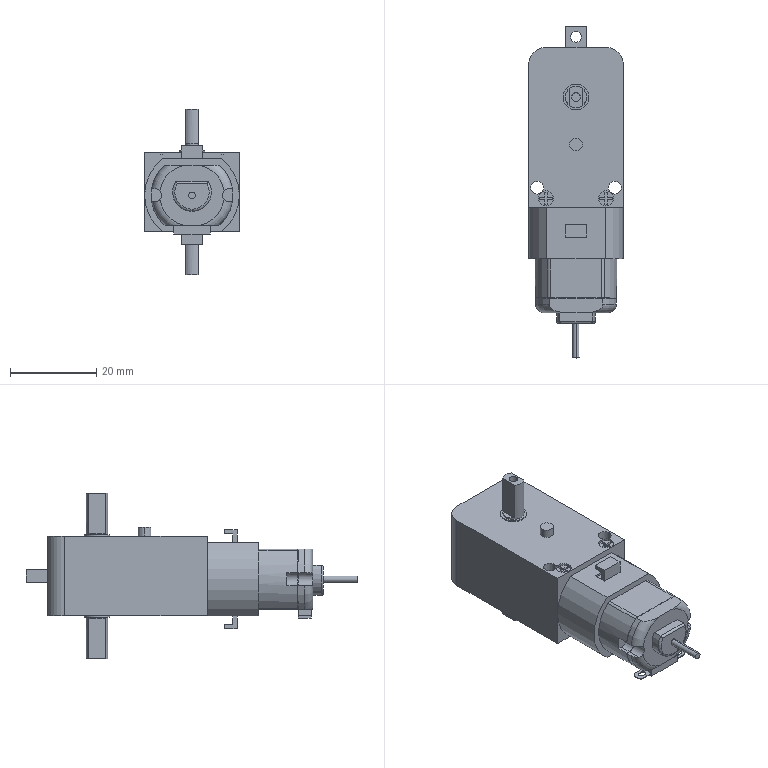Part | SolidWorks | features ICE 23, Fillet 5, Extrusion 1, RevCut 1 | 7 solids | 201 faces | box 22 x 77 x 38.5 mm | volume 22035 mm3 | plane 126 | cylinder 63 | torus 6 | cone 6 | commonest cylinder face diameters 2 x12 3 x10 5 x8 1.285 x6 3.5 x6 18.25 x6